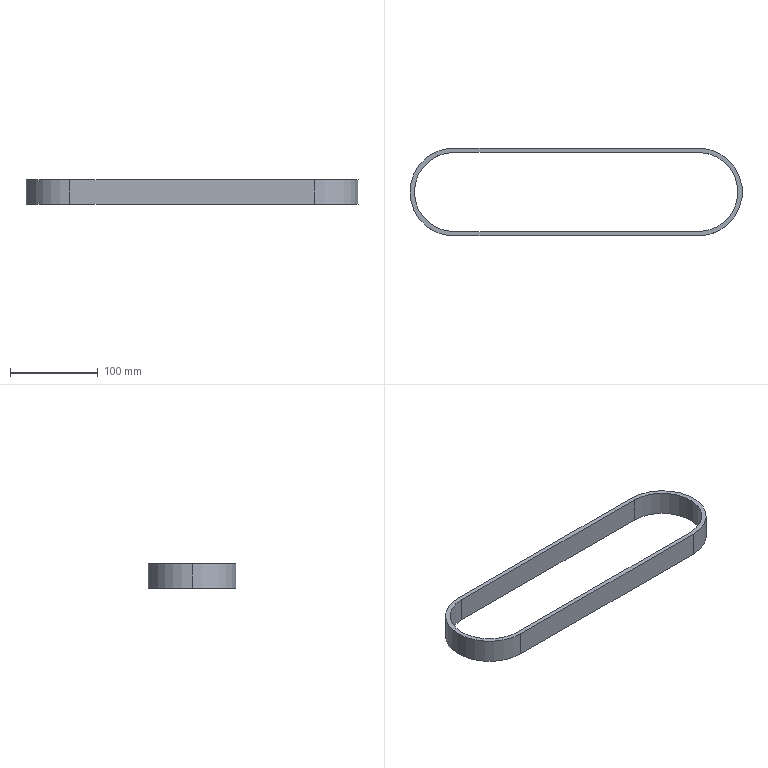Part | SolidWorks | features Extrusion 1 | 1 solid | 12 faces | box 378 x 100 x 28 mm | volume 119623 mm3 | cylinder 6 | plane 6 | commonest cylinder face diameters 90 x3 100 x3
STEP:
#1=CARTESIAN_POINT('',(0.,45.,28.));
#2=VERTEX_POINT('',#1);
#3=CARTESIAN_POINT('',(-45.,0.,28.));
#4=VERTEX_POINT('',#3);
#5=CARTESIAN_POINT('',(0.,0.,28.));
#6=DIRECTION('',(0.,0.,1.));
#7=DIRECTION('',(1.,0.,0.));
#8=AXIS2_PLACEMENT_3D('',#5,#6,#7);
#9=CIRCLE('',#8,45.);
#10=EDGE_CURVE('',#2,#4,#9,.T.);
#11=ORIENTED_EDGE('',*,*,#10,.T.);
#12=CARTESIAN_POINT('',(-45.,0.,0.));
#13=VERTEX_POINT('',#12);
#14=CARTESIAN_POINT('',(-45.,0.,28.));
#15=DIRECTION('',(0.,0.,-1.));
#16=VECTOR('',#15,1000.);
#17=LINE('',#14,#16);
#18=EDGE_CURVE('',#4,#13,#17,.T.);
#19=ORIENTED_EDGE('',*,*,#18,.T.);
#20=CARTESIAN_POINT('',(0.,45.,0.));
#21=VERTEX_POINT('',#20);
#22=CARTESIAN_POINT('',(0.,0.,0.));
#23=DIRECTION('',(0.,0.,1.));
#24=DIRECTION('',(1.,0.,0.));
#25=AXIS2_PLACEMENT_3D('',#22,#23,#24);
#26=CIRCLE('',#25,45.);
#27=EDGE_CURVE('',#21,#13,#26,.T.);
#28=ORIENTED_EDGE('',*,*,#27,.F.);
#29=CARTESIAN_POINT('',(0.,45.,28.));
#30=DIRECTION('',(0.,0.,-1.));
#31=VECTOR('',#30,1000.);
#32=LINE('',#29,#31);
#33=EDGE_CURVE('',#2,#21,#32,.T.);
#34=ORIENTED_EDGE('',*,*,#33,.F.);
#35=EDGE_LOOP('',(#11,#19,#28,#34));
#36=FACE_OUTER_BOUND('',#35,.T.);
#37=CARTESIAN_POINT('',(0.,0.,28.));
#38=DIRECTION('',(0.,0.,-1.));
#39=DIRECTION('',(-1.,0.,0.));
#40=AXIS2_PLACEMENT_3D('',#37,#38,#39);
#41=CYLINDRICAL_SURFACE('',#40,45.);
#42=ADVANCED_FACE('',(#36),#41,.F.);
#43=CARTESIAN_POINT('',(-50.,0.,28.));
#44=VERTEX_POINT('',#43);
#45=CARTESIAN_POINT('',(0.,-50.,28.));
#46=VERTEX_POINT('',#45);
#47=CARTESIAN_POINT('',(0.,0.,28.));
#48=DIRECTION('',(0.,0.,1.));
#49=DIRECTION('',(1.,0.,0.));
#50=AXIS2_PLACEMENT_3D('',#47,#48,#49);
#51=CIRCLE('',#50,50.);
#52=EDGE_CURVE('',#44,#46,#51,.T.);
#53=ORIENTED_EDGE('',*,*,#52,.F.);
#54=CARTESIAN_POINT('',(-50.,0.,0.));
#55=VERTEX_POINT('',#54);
#56=CARTESIAN_POINT('',(-50.,0.,28.));
#57=DIRECTION('',(0.,0.,-1.));
#58=VECTOR('',#57,1000.);
#59=LINE('',#56,#58);
#60=EDGE_CURVE('',#44,#55,#59,.T.);
#61=ORIENTED_EDGE('',*,*,#60,.T.);
#62=CARTESIAN_POINT('',(0.,-50.,0.));
#63=VERTEX_POINT('',#62);
#64=CARTESIAN_POINT('',(0.,0.,0.));
#65=DIRECTION('',(0.,0.,1.));
#66=DIRECTION('',(1.,0.,0.));
#67=AXIS2_PLACEMENT_3D('',#64,#65,#66);
#68=CIRCLE('',#67,50.);
#69=EDGE_CURVE('',#55,#63,#68,.T.);
#70=ORIENTED_EDGE('',*,*,#69,.T.);
#71=CARTESIAN_POINT('',(0.,-50.,28.));
#72=DIRECTION('',(0.,0.,-1.));
#73=VECTOR('',#72,1000.);
#74=LINE('',#71,#73);
#75=EDGE_CURVE('',#46,#63,#74,.T.);
#76=ORIENTED_EDGE('',*,*,#75,.F.);
#77=EDGE_LOOP('',(#53,#61,#70,#76));
#78=FACE_OUTER_BOUND('',#77,.T.);
#79=CARTESIAN_POINT('',(0.,0.,28.));
#80=DIRECTION('',(0.,0.,-1.));
#81=DIRECTION('',(-1.,0.,0.));
#82=AXIS2_PLACEMENT_3D('',#79,#80,#81);
#83=CYLINDRICAL_SURFACE('',#82,50.);
#84=ADVANCED_FACE('',(#78),#83,.T.);
#85=CARTESIAN_POINT('',(0.,50.,28.));
#86=VERTEX_POINT('',#85);
#87=CARTESIAN_POINT('',(0.,0.,28.));
#88=DIRECTION('',(0.,0.,1.));
#89=DIRECTION('',(1.,0.,0.));
#90=AXIS2_PLACEMENT_3D('',#87,#88,#89);
#91=CIRCLE('',#90,50.);
#92=EDGE_CURVE('',#86,#44,#91,.T.);
#93=ORIENTED_EDGE('',*,*,#92,.T.);
#94=ORIENTED_EDGE('',*,*,#52,.T.);
#95=CARTESIAN_POINT('',(278.,-50.,28.));
#96=VERTEX_POINT('',#95);
#97=CARTESIAN_POINT('',(0.,-50.,28.));
#98=DIRECTION('',(1.,0.,0.));
#99=VECTOR('',#98,1000.);
#100=LINE('',#97,#99);
#101=EDGE_CURVE('',#46,#96,#100,.T.);
#102=ORIENTED_EDGE('',*,*,#101,.T.);
#103=CARTESIAN_POINT('',(278.,50.,28.));
#104=VERTEX_POINT('',#103);
#105=CARTESIAN_POINT('',(278.,0.,28.));
#106=DIRECTION('',(0.,0.,1.));
#107=DIRECTION('',(1.,0.,0.));
#108=AXIS2_PLACEMENT_3D('',#105,#106,#107);
#109=CIRCLE('',#108,50.);
#110=EDGE_CURVE('',#96,#104,#109,.T.);
#111=ORIENTED_EDGE('',*,*,#110,.T.);
#112=CARTESIAN_POINT('',(0.,50.,28.));
#113=DIRECTION('',(-1.,0.,0.));
#114=VECTOR('',#113,1000.);
#115=LINE('',#112,#114);
#116=EDGE_CURVE('',#104,#86,#115,.T.);
#117=ORIENTED_EDGE('',*,*,#116,.T.);
#118=EDGE_LOOP('',(#93,#94,#102,#111,#117));
#119=FACE_OUTER_BOUND('',#118,.T.);
#120=CARTESIAN_POINT('',(0.,-45.,28.));
#121=VERTEX_POINT('',#120);
#122=CARTESIAN_POINT('',(278.,-45.,28.));
#123=VERTEX_POINT('',#122);
#124=CARTESIAN_POINT('',(0.,-45.,28.));
#125=DIRECTION('',(1.,0.,0.));
#126=VECTOR('',#125,1000.);
#127=LINE('',#124,#126);
#128=EDGE_CURVE('',#121,#123,#127,.T.);
#129=ORIENTED_EDGE('',*,*,#128,.F.);
#130=CARTESIAN_POINT('',(0.,0.,28.));
#131=DIRECTION('',(0.,0.,1.));
#132=DIRECTION('',(1.,0.,0.));
#133=AXIS2_PLACEMENT_3D('',#130,#131,#132);
#134=CIRCLE('',#133,45.);
#135=EDGE_CURVE('',#4,#121,#134,.T.);
#136=ORIENTED_EDGE('',*,*,#135,.F.);
#137=ORIENTED_EDGE('',*,*,#10,.F.);
#138=CARTESIAN_POINT('',(278.,45.,28.));
#139=VERTEX_POINT('',#138);
#140=CARTESIAN_POINT('',(0.,45.,28.));
#141=DIRECTION('',(-1.,0.,0.));
#142=VECTOR('',#141,1000.);
#143=LINE('',#140,#142);
#144=EDGE_CURVE('',#139,#2,#143,.T.);
#145=ORIENTED_EDGE('',*,*,#144,.F.);
#146=CARTESIAN_POINT('',(278.,0.,28.));
#147=DIRECTION('',(0.,0.,1.));
#148=DIRECTION('',(1.,0.,0.));
#149=AXIS2_PLACEMENT_3D('',#146,#147,#148);
#150=CIRCLE('',#149,45.);
#151=EDGE_CURVE('',#123,#139,#150,.T.);
#152=ORIENTED_EDGE('',*,*,#151,.F.);
#153=EDGE_LOOP('',(#129,#136,#137,#145,#152));
#154=FACE_BOUND('',#153,.T.);
#155=CARTESIAN_POINT('',(0.,0.,28.));
#156=DIRECTION('',(0.,0.,1.));
#157=DIRECTION('',(1.,0.,0.));
#158=AXIS2_PLACEMENT_3D('',#155,#156,#157);
#159=PLANE('',#158);
#160=ADVANCED_FACE('',(#119,#154),#159,.T.);
#161=CARTESIAN_POINT('',(0.,50.,0.));
#162=VERTEX_POINT('',#161);
#163=CARTESIAN_POINT('',(0.,0.,0.));
#164=DIRECTION('',(0.,0.,1.));
#165=DIRECTION('',(1.,0.,0.));
#166=AXIS2_PLACEMENT_3D('',#163,#164,#165);
#167=CIRCLE('',#166,50.);
#168=EDGE_CURVE('',#162,#55,#167,.T.);
#169=ORIENTED_EDGE('',*,*,#168,.F.);
#170=CARTESIAN_POINT('',(278.,50.,0.));
#171=VERTEX_POINT('',#170);
#172=CARTESIAN_POINT('',(0.,50.,0.));
#173=DIRECTION('',(-1.,0.,0.));
#174=VECTOR('',#173,1000.);
#175=LINE('',#172,#174);
#176=EDGE_CURVE('',#171,#162,#175,.T.);
#177=ORIENTED_EDGE('',*,*,#176,.F.);
#178=CARTESIAN_POINT('',(278.,-50.,0.));
#179=VERTEX_POINT('',#178);
#180=CARTESIAN_POINT('',(278.,0.,0.));
#181=DIRECTION('',(0.,0.,1.));
#182=DIRECTION('',(1.,0.,0.));
#183=AXIS2_PLACEMENT_3D('',#180,#181,#182);
#184=CIRCLE('',#183,50.);
#185=EDGE_CURVE('',#179,#171,#184,.T.);
#186=ORIENTED_EDGE('',*,*,#185,.F.);
#187=CARTESIAN_POINT('',(0.,-50.,0.));
#188=DIRECTION('',(1.,0.,0.));
#189=VECTOR('',#188,1000.);
#190=LINE('',#187,#189);
#191=EDGE_CURVE('',#63,#179,#190,.T.);
#192=ORIENTED_EDGE('',*,*,#191,.F.);
#193=ORIENTED_EDGE('',*,*,#69,.F.);
#194=EDGE_LOOP('',(#169,#177,#186,#192,#193));
#195=FACE_OUTER_BOUND('',#194,.T.);
#196=ORIENTED_EDGE('',*,*,#27,.T.);
#197=CARTESIAN_POINT('',(0.,-45.,0.));
#198=VERTEX_POINT('',#197);
#199=CARTESIAN_POINT('',(0.,0.,0.));
#200=DIRECTION('',(0.,0.,1.));
#201=DIRECTION('',(1.,0.,0.));
#202=AXIS2_PLACEMENT_3D('',#199,#200,#201);
#203=CIRCLE('',#202,45.);
#204=EDGE_CURVE('',#13,#198,#203,.T.);
#205=ORIENTED_EDGE('',*,*,#204,.T.);
#206=CARTESIAN_POINT('',(278.,-45.,0.));
#207=VERTEX_POINT('',#206);
#208=CARTESIAN_POINT('',(0.,-45.,0.));
#209=DIRECTION('',(1.,0.,0.));
#210=VECTOR('',#209,1000.);
#211=LINE('',#208,#210);
#212=EDGE_CURVE('',#198,#207,#211,.T.);
#213=ORIENTED_EDGE('',*,*,#212,.T.);
#214=CARTESIAN_POINT('',(278.,45.,0.));
#215=VERTEX_POINT('',#214);
#216=CARTESIAN_POINT('',(278.,0.,0.));
#217=DIRECTION('',(0.,0.,1.));
#218=DIRECTION('',(1.,0.,0.));
#219=AXIS2_PLACEMENT_3D('',#216,#217,#218);
#220=CIRCLE('',#219,45.);
#221=EDGE_CURVE('',#207,#215,#220,.T.);
#222=ORIENTED_EDGE('',*,*,#221,.T.);
#223=CARTESIAN_POINT('',(0.,45.,0.));
#224=DIRECTION('',(-1.,0.,0.));
#225=VECTOR('',#224,1000.);
#226=LINE('',#223,#225);
#227=EDGE_CURVE('',#215,#21,#226,.T.);
#228=ORIENTED_EDGE('',*,*,#227,.T.);
#229=EDGE_LOOP('',(#196,#205,#213,#222,#228));
#230=FACE_BOUND('',#229,.T.);
#231=CARTESIAN_POINT('',(0.,0.,0.));
#232=DIRECTION('',(0.,0.,1.));
#233=DIRECTION('',(1.,0.,0.));
#234=AXIS2_PLACEMENT_3D('',#231,#232,#233);
#235=PLANE('',#234);
#236=ADVANCED_FACE('',(#195,#230),#235,.F.);
#237=ORIENTED_EDGE('',*,*,#60,.F.);
#238=ORIENTED_EDGE('',*,*,#92,.F.);
#239=CARTESIAN_POINT('',(0.,50.,28.));
#240=DIRECTION('',(0.,0.,-1.));
#241=VECTOR('',#240,1000.);
#242=LINE('',#239,#241);
#243=EDGE_CURVE('',#86,#162,#242,.T.);
#244=ORIENTED_EDGE('',*,*,#243,.T.);
#245=ORIENTED_EDGE('',*,*,#168,.T.);
#246=EDGE_LOOP('',(#237,#238,#244,#245));
#247=FACE_OUTER_BOUND('',#246,.T.);
#248=CARTESIAN_POINT('',(0.,0.,28.));
#249=DIRECTION('',(0.,0.,-1.));
#250=DIRECTION('',(-1.,0.,0.));
#251=AXIS2_PLACEMENT_3D('',#248,#249,#250);
#252=CYLINDRICAL_SURFACE('',#251,50.);
#253=ADVANCED_FACE('',(#247),#252,.T.);
#254=ORIENTED_EDGE('',*,*,#191,.T.);
#255=CARTESIAN_POINT('',(278.,-50.,28.));
#256=DIRECTION('',(0.,0.,-1.));
#257=VECTOR('',#256,1000.);
#258=LINE('',#255,#257);
#259=EDGE_CURVE('',#96,#179,#258,.T.);
#260=ORIENTED_EDGE('',*,*,#259,.F.);
#261=ORIENTED_EDGE('',*,*,#101,.F.);
#262=ORIENTED_EDGE('',*,*,#75,.T.);
#263=EDGE_LOOP('',(#254,#260,#261,#262));
#264=FACE_OUTER_BOUND('',#263,.T.);
#265=CARTESIAN_POINT('',(0.,-50.,28.));
#266=DIRECTION('',(0.,1.,0.));
#267=DIRECTION('',(0.,0.,1.));
#268=AXIS2_PLACEMENT_3D('',#265,#266,#267);
#269=PLANE('',#268);
#270=ADVANCED_FACE('',(#264),#269,.F.);
#271=ORIENTED_EDGE('',*,*,#185,.T.);
#272=CARTESIAN_POINT('',(278.,50.,28.));
#273=DIRECTION('',(0.,0.,-1.));
#274=VECTOR('',#273,1000.);
#275=LINE('',#272,#274);
#276=EDGE_CURVE('',#104,#171,#275,.T.);
#277=ORIENTED_EDGE('',*,*,#276,.F.);
#278=ORIENTED_EDGE('',*,*,#110,.F.);
#279=ORIENTED_EDGE('',*,*,#259,.T.);
#280=EDGE_LOOP('',(#271,#277,#278,#279));
#281=FACE_OUTER_BOUND('',#280,.T.);
#282=CARTESIAN_POINT('',(278.,0.,28.));
#283=DIRECTION('',(0.,0.,-1.));
#284=DIRECTION('',(-1.,0.,0.));
#285=AXIS2_PLACEMENT_3D('',#282,#283,#284);
#286=CYLINDRICAL_SURFACE('',#285,50.);
#287=ADVANCED_FACE('',(#281),#286,.T.);
#288=ORIENTED_EDGE('',*,*,#176,.T.);
#289=ORIENTED_EDGE('',*,*,#243,.F.);
#290=ORIENTED_EDGE('',*,*,#116,.F.);
#291=ORIENTED_EDGE('',*,*,#276,.T.);
#292=EDGE_LOOP('',(#288,#289,#290,#291));
#293=FACE_OUTER_BOUND('',#292,.T.);
#294=CARTESIAN_POINT('',(0.,50.,28.));
#295=DIRECTION('',(0.,-1.,0.));
#296=DIRECTION('',(0.,0.,-1.));
#297=AXIS2_PLACEMENT_3D('',#294,#295,#296);
#298=PLANE('',#297);
#299=ADVANCED_FACE('',(#293),#298,.F.);
#300=ORIENTED_EDGE('',*,*,#18,.F.);
#301=ORIENTED_EDGE('',*,*,#135,.T.);
#302=CARTESIAN_POINT('',(0.,-45.,28.));
#303=DIRECTION('',(0.,0.,-1.));
#304=VECTOR('',#303,1000.);
#305=LINE('',#302,#304);
#306=EDGE_CURVE('',#121,#198,#305,.T.);
#307=ORIENTED_EDGE('',*,*,#306,.T.);
#308=ORIENTED_EDGE('',*,*,#204,.F.);
#309=EDGE_LOOP('',(#300,#301,#307,#308));
#310=FACE_OUTER_BOUND('',#309,.T.);
#311=CARTESIAN_POINT('',(0.,0.,28.));
#312=DIRECTION('',(0.,0.,-1.));
#313=DIRECTION('',(-1.,0.,0.));
#314=AXIS2_PLACEMENT_3D('',#311,#312,#313);
#315=CYLINDRICAL_SURFACE('',#314,45.);
#316=ADVANCED_FACE('',(#310),#315,.F.);
#317=ORIENTED_EDGE('',*,*,#212,.F.);
#318=ORIENTED_EDGE('',*,*,#306,.F.);
#319=ORIENTED_EDGE('',*,*,#128,.T.);
#320=CARTESIAN_POINT('',(278.,-45.,28.));
#321=DIRECTION('',(0.,0.,-1.));
#322=VECTOR('',#321,1000.);
#323=LINE('',#320,#322);
#324=EDGE_CURVE('',#123,#207,#323,.T.);
#325=ORIENTED_EDGE('',*,*,#324,.T.);
#326=EDGE_LOOP('',(#317,#318,#319,#325));
#327=FACE_OUTER_BOUND('',#326,.T.);
#328=CARTESIAN_POINT('',(0.,-45.,28.));
#329=DIRECTION('',(0.,1.,0.));
#330=DIRECTION('',(0.,0.,1.));
#331=AXIS2_PLACEMENT_3D('',#328,#329,#330);
#332=PLANE('',#331);
#333=ADVANCED_FACE('',(#327),#332,.T.);
#334=ORIENTED_EDGE('',*,*,#221,.F.);
#335=ORIENTED_EDGE('',*,*,#324,.F.);
#336=ORIENTED_EDGE('',*,*,#151,.T.);
#337=CARTESIAN_POINT('',(278.,45.,28.));
#338=DIRECTION('',(0.,0.,-1.));
#339=VECTOR('',#338,1000.);
#340=LINE('',#337,#339);
#341=EDGE_CURVE('',#139,#215,#340,.T.);
#342=ORIENTED_EDGE('',*,*,#341,.T.);
#343=EDGE_LOOP('',(#334,#335,#336,#342));
#344=FACE_OUTER_BOUND('',#343,.T.);
#345=CARTESIAN_POINT('',(278.,0.,28.));
#346=DIRECTION('',(0.,0.,-1.));
#347=DIRECTION('',(-1.,0.,0.));
#348=AXIS2_PLACEMENT_3D('',#345,#346,#347);
#349=CYLINDRICAL_SURFACE('',#348,45.);
#350=ADVANCED_FACE('',(#344),#349,.F.);
#351=ORIENTED_EDGE('',*,*,#227,.F.);
#352=ORIENTED_EDGE('',*,*,#341,.F.);
#353=ORIENTED_EDGE('',*,*,#144,.T.);
#354=ORIENTED_EDGE('',*,*,#33,.T.);
#355=EDGE_LOOP('',(#351,#352,#353,#354));
#356=FACE_OUTER_BOUND('',#355,.T.);
#357=CARTESIAN_POINT('',(0.,45.,28.));
#358=DIRECTION('',(0.,-1.,0.));
#359=DIRECTION('',(0.,0.,-1.));
#360=AXIS2_PLACEMENT_3D('',#357,#358,#359);
#361=PLANE('',#360);
#362=ADVANCED_FACE('',(#356),#361,.T.);
#363=CLOSED_SHELL('',(#42,#84,#160,#236,#253,#270,#287,#299,#316,#333,#350,#362));
#364=MANIFOLD_SOLID_BREP('',#363);
#365=CARTESIAN_POINT('',(0.,0.,0.));
#366=DIRECTION('',(0.,0.,1.));
#367=DIRECTION('',(1.,0.,0.));
#368=AXIS2_PLACEMENT_3D('',#365,#366,#367);
#369=(LENGTH_UNIT()NAMED_UNIT(*)SI_UNIT(.MILLI.,.METRE.));
#370=UNCERTAINTY_MEASURE_WITH_UNIT(LENGTH_MEASURE(0.00001),#369,'','');
#371=(NAMED_UNIT(*)PLANE_ANGLE_UNIT()SI_UNIT($,.RADIAN.));
#372=(NAMED_UNIT(*)SI_UNIT($,.STERADIAN.)SOLID_ANGLE_UNIT());
#373=(GEOMETRIC_REPRESENTATION_CONTEXT(3)GLOBAL_UNCERTAINTY_ASSIGNED_CONTEXT((#370))GLOBAL_UNIT_ASSIGNED_CONTEXT((#369,#371,#372))REPRESENTATION_CONTEXT('',''));
#374=ADVANCED_BREP_SHAPE_REPRESENTATION('',(#364,#368),#373);